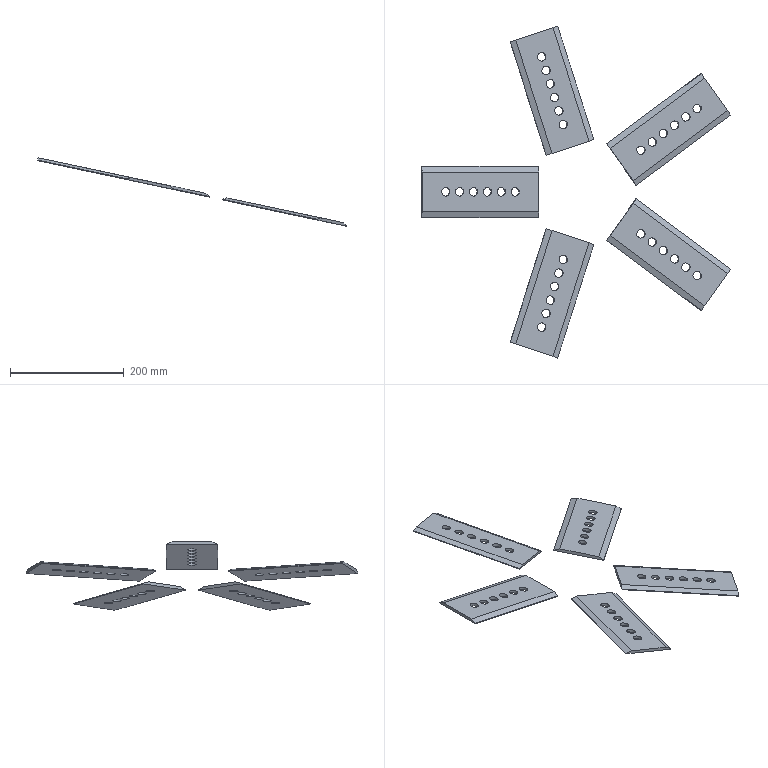Part | STEP file | HL4GZ-1.862.632 (blade) | 5 solids | 70 faces | box 543.655 x 584.18 x 120.404 mm | volume 403993 mm3 | plane 40 | cylinder 30 | commonest cylinder face diameters 15 x30